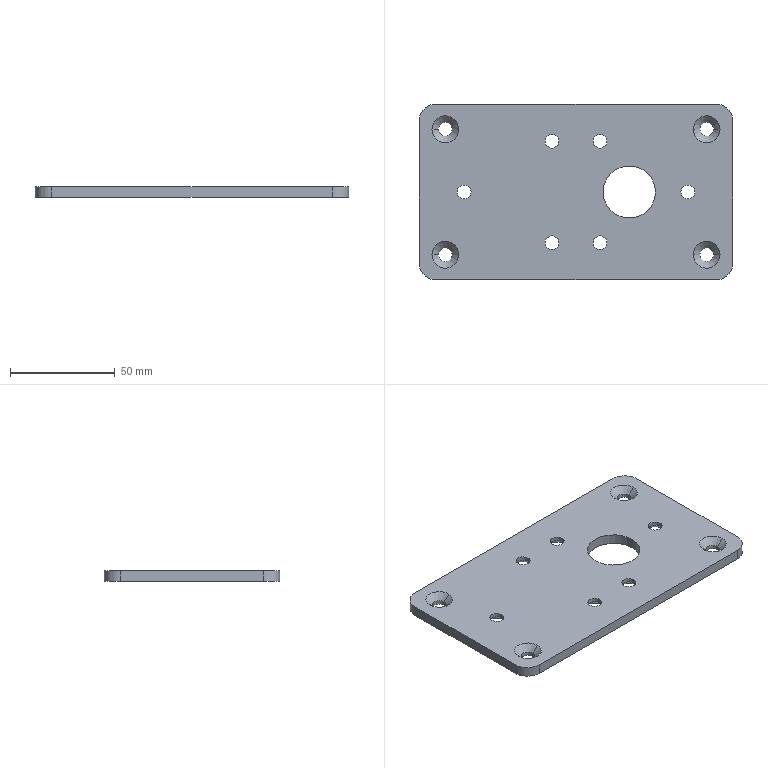Part | STEP file | Gear box SGN-5-03 | 1 solid | 52 faces | box 150 x 84 x 5 mm | volume 57252 mm3 | cylinder 26 | cone 20 | plane 6 | commonest cylinder face diameters 6.6 x20 16 x4 25 x2